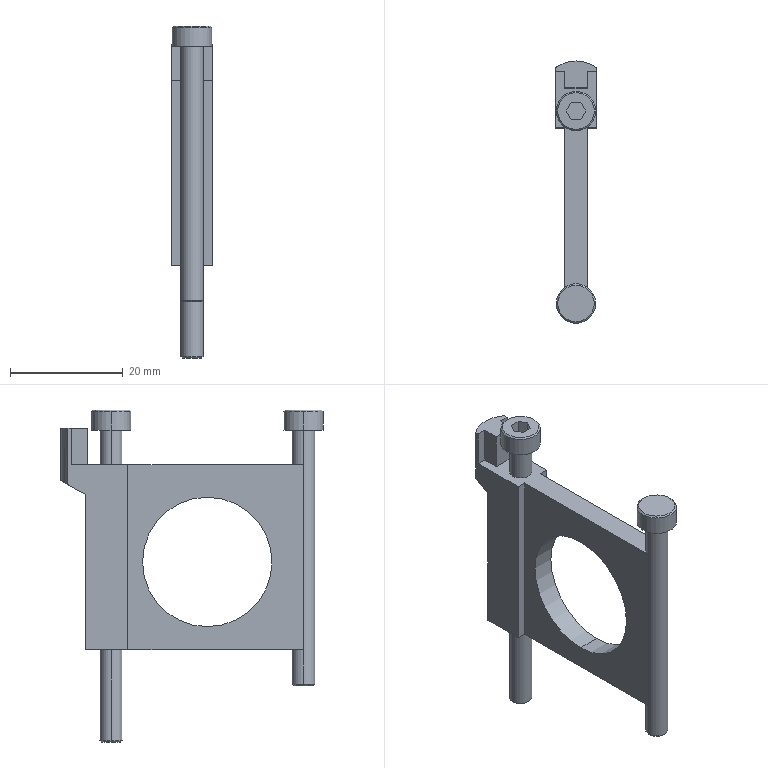Part | STEP file | Y300T_Y3035DB Interface_3 | 1 solid | 51 faces | box 7.2 x 46.6 x 59 mm | volume 5410 mm3 | plane 29 | cylinder 14 | cone 8 | commonest cylinder face diameters 4 x7 7 x4 23 x2 12 x1
STEP:
#1=CARTESIAN_POINT('',(-1.75,17.1,-32.));
#2=VERTEX_POINT('',#1);
#3=CARTESIAN_POINT('',(1.75,17.1,-32.));
#4=VERTEX_POINT('',#3);
#5=CARTESIAN_POINT('',(0.,17.1,-32.));
#6=DIRECTION('',(0.,0.,-1.));
#7=DIRECTION('',(1.,0.,0.));
#8=AXIS2_PLACEMENT_3D('',#5,#6,#7);
#9=CIRCLE('',#8,1.75);
#10=EDGE_CURVE('',#2,#4,#9,.T.);
#11=ORIENTED_EDGE('',*,*,#10,.F.);
#12=CARTESIAN_POINT('',(-2.,17.1,-31.75));
#13=VERTEX_POINT('',#12);
#14=CARTESIAN_POINT('',(-2.,17.1,-31.75));
#15=DIRECTION('',(-0.7071,0.,0.7071));
#16=VECTOR('',#15,1000.);
#17=LINE('',#14,#16);
#18=EDGE_CURVE('',#2,#13,#17,.T.);
#19=ORIENTED_EDGE('',*,*,#18,.T.);
#20=CARTESIAN_POINT('',(2.,17.1,-31.75));
#21=VERTEX_POINT('',#20);
#22=CARTESIAN_POINT('',(0.,17.1,-31.75));
#23=DIRECTION('',(0.,0.,1.));
#24=DIRECTION('',(1.,0.,0.));
#25=AXIS2_PLACEMENT_3D('',#22,#23,#24);
#26=CIRCLE('',#25,2.);
#27=EDGE_CURVE('',#21,#13,#26,.T.);
#28=ORIENTED_EDGE('',*,*,#27,.F.);
#29=CARTESIAN_POINT('',(2.,17.1,-31.75));
#30=DIRECTION('',(0.7071,0.,0.7071));
#31=VECTOR('',#30,1000.);
#32=LINE('',#29,#31);
#33=EDGE_CURVE('',#4,#21,#32,.T.);
#34=ORIENTED_EDGE('',*,*,#33,.F.);
#35=EDGE_LOOP('',(#11,#19,#28,#34));
#36=FACE_OUTER_BOUND('',#35,.T.);
#37=CARTESIAN_POINT('',(0.,17.1,-31.75));
#38=DIRECTION('',(0.,0.,1.));
#39=DIRECTION('',(1.,0.,0.));
#40=AXIS2_PLACEMENT_3D('',#37,#38,#39);
#41=CONICAL_SURFACE('',#40,2.,0.7854);
#42=ADVANCED_FACE('',(#36),#41,.T.);
#43=CARTESIAN_POINT('',(-1.75,-17.1,-22.));
#44=VERTEX_POINT('',#43);
#45=CARTESIAN_POINT('',(1.75,-17.1,-22.));
#46=VERTEX_POINT('',#45);
#47=CARTESIAN_POINT('',(0.,-17.1,-22.));
#48=DIRECTION('',(0.,0.,-1.));
#49=DIRECTION('',(1.,0.,0.));
#50=AXIS2_PLACEMENT_3D('',#47,#48,#49);
#51=CIRCLE('',#50,1.75);
#52=EDGE_CURVE('',#44,#46,#51,.T.);
#53=ORIENTED_EDGE('',*,*,#52,.F.);
#54=CARTESIAN_POINT('',(-2.,-17.1,-21.75));
#55=VERTEX_POINT('',#54);
#56=CARTESIAN_POINT('',(-2.,-17.1,-21.75));
#57=DIRECTION('',(-0.7071,0.,0.7071));
#58=VECTOR('',#57,1000.);
#59=LINE('',#56,#58);
#60=EDGE_CURVE('',#44,#55,#59,.T.);
#61=ORIENTED_EDGE('',*,*,#60,.T.);
#62=CARTESIAN_POINT('',(2.,-17.1,-21.75));
#63=VERTEX_POINT('',#62);
#64=CARTESIAN_POINT('',(0.,-17.1,-21.75));
#65=DIRECTION('',(0.,0.,1.));
#66=DIRECTION('',(1.,0.,0.));
#67=AXIS2_PLACEMENT_3D('',#64,#65,#66);
#68=CIRCLE('',#67,2.);
#69=EDGE_CURVE('',#63,#55,#68,.T.);
#70=ORIENTED_EDGE('',*,*,#69,.F.);
#71=CARTESIAN_POINT('',(2.,-17.1,-21.75));
#72=DIRECTION('',(0.7071,0.,0.7071));
#73=VECTOR('',#72,1000.);
#74=LINE('',#71,#73);
#75=EDGE_CURVE('',#46,#63,#74,.T.);
#76=ORIENTED_EDGE('',*,*,#75,.F.);
#77=EDGE_LOOP('',(#53,#61,#70,#76));
#78=FACE_OUTER_BOUND('',#77,.T.);
#79=CARTESIAN_POINT('',(0.,-17.1,-21.75));
#80=DIRECTION('',(0.,0.,1.));
#81=DIRECTION('',(1.,0.,0.));
#82=AXIS2_PLACEMENT_3D('',#79,#80,#81);
#83=CONICAL_SURFACE('',#82,2.,0.7854);
#84=ADVANCED_FACE('',(#78),#83,.T.);
#85=CARTESIAN_POINT('',(3.25,-17.1,27.));
#86=VERTEX_POINT('',#85);
#87=CARTESIAN_POINT('',(-3.25,-17.1,27.));
#88=VERTEX_POINT('',#87);
#89=CARTESIAN_POINT('',(0.,-17.1,27.));
#90=DIRECTION('',(0.,0.,1.));
#91=DIRECTION('',(-1.,0.,0.));
#92=AXIS2_PLACEMENT_3D('',#89,#90,#91);
#93=CIRCLE('',#92,3.25);
#94=EDGE_CURVE('',#86,#88,#93,.T.);
#95=ORIENTED_EDGE('',*,*,#94,.F.);
#96=CARTESIAN_POINT('',(3.5,-17.1,26.75));
#97=VERTEX_POINT('',#96);
#98=CARTESIAN_POINT('',(3.25,-17.1,27.));
#99=DIRECTION('',(0.7071,0.,-0.7071));
#100=VECTOR('',#99,1000.);
#101=LINE('',#98,#100);
#102=EDGE_CURVE('',#86,#97,#101,.T.);
#103=ORIENTED_EDGE('',*,*,#102,.T.);
#104=CARTESIAN_POINT('',(-3.5,-17.1,26.75));
#105=VERTEX_POINT('',#104);
#106=CARTESIAN_POINT('',(0.,-17.1,26.75));
#107=DIRECTION('',(0.,0.,-1.));
#108=DIRECTION('',(-1.,0.,0.));
#109=AXIS2_PLACEMENT_3D('',#106,#107,#108);
#110=CIRCLE('',#109,3.5);
#111=EDGE_CURVE('',#105,#97,#110,.T.);
#112=ORIENTED_EDGE('',*,*,#111,.F.);
#113=CARTESIAN_POINT('',(-3.25,-17.1,27.));
#114=DIRECTION('',(-0.7071,0.,-0.7071));
#115=VECTOR('',#114,1000.);
#116=LINE('',#113,#115);
#117=EDGE_CURVE('',#88,#105,#116,.T.);
#118=ORIENTED_EDGE('',*,*,#117,.F.);
#119=EDGE_LOOP('',(#95,#103,#112,#118));
#120=FACE_OUTER_BOUND('',#119,.T.);
#121=CARTESIAN_POINT('',(0.,-17.1,27.));
#122=DIRECTION('',(0.,0.,-1.));
#123=DIRECTION('',(-1.,0.,0.));
#124=AXIS2_PLACEMENT_3D('',#121,#122,#123);
#125=CONICAL_SURFACE('',#124,3.25,0.7854);
#126=ADVANCED_FACE('',(#120),#125,.T.);
#127=CARTESIAN_POINT('',(3.25,17.1,27.));
#128=VERTEX_POINT('',#127);
#129=CARTESIAN_POINT('',(-3.25,17.1,27.));
#130=VERTEX_POINT('',#129);
#131=CARTESIAN_POINT('',(0.,17.1,27.));
#132=DIRECTION('',(0.,0.,1.));
#133=DIRECTION('',(-1.,0.,0.));
#134=AXIS2_PLACEMENT_3D('',#131,#132,#133);
#135=CIRCLE('',#134,3.25);
#136=EDGE_CURVE('',#128,#130,#135,.T.);
#137=ORIENTED_EDGE('',*,*,#136,.F.);
#138=CARTESIAN_POINT('',(3.5,17.1,26.75));
#139=VERTEX_POINT('',#138);
#140=CARTESIAN_POINT('',(3.25,17.1,27.));
#141=DIRECTION('',(0.7071,0.,-0.7071));
#142=VECTOR('',#141,1000.);
#143=LINE('',#140,#142);
#144=EDGE_CURVE('',#128,#139,#143,.T.);
#145=ORIENTED_EDGE('',*,*,#144,.T.);
#146=CARTESIAN_POINT('',(-3.5,17.1,26.75));
#147=VERTEX_POINT('',#146);
#148=CARTESIAN_POINT('',(0.,17.1,26.75));
#149=DIRECTION('',(0.,0.,-1.));
#150=DIRECTION('',(-1.,0.,0.));
#151=AXIS2_PLACEMENT_3D('',#148,#149,#150);
#152=CIRCLE('',#151,3.5);
#153=EDGE_CURVE('',#147,#139,#152,.T.);
#154=ORIENTED_EDGE('',*,*,#153,.F.);
#155=CARTESIAN_POINT('',(-3.25,17.1,27.));
#156=DIRECTION('',(-0.7071,0.,-0.7071));
#157=VECTOR('',#156,1000.);
#158=LINE('',#155,#157);
#159=EDGE_CURVE('',#130,#147,#158,.T.);
#160=ORIENTED_EDGE('',*,*,#159,.F.);
#161=EDGE_LOOP('',(#137,#145,#154,#160));
#162=FACE_OUTER_BOUND('',#161,.T.);
#163=CARTESIAN_POINT('',(0.,17.1,27.));
#164=DIRECTION('',(0.,0.,-1.));
#165=DIRECTION('',(-1.,0.,0.));
#166=AXIS2_PLACEMENT_3D('',#163,#164,#165);
#167=CONICAL_SURFACE('',#166,3.25,0.7854);
#168=ADVANCED_FACE('',(#162),#167,.T.);
#169=ORIENTED_EDGE('',*,*,#69,.T.);
#170=CARTESIAN_POINT('',(-2.,-17.1,-15.6));
#171=VERTEX_POINT('',#170);
#172=CARTESIAN_POINT('',(-2.,-17.1,32.925));
#173=DIRECTION('',(0.,0.,1.));
#174=VECTOR('',#173,1000.);
#175=LINE('',#172,#174);
#176=EDGE_CURVE('',#55,#171,#175,.T.);
#177=ORIENTED_EDGE('',*,*,#176,.T.);
#178=CARTESIAN_POINT('',(2.,-17.1,-15.6));
#179=VERTEX_POINT('',#178);
#180=CARTESIAN_POINT('',(0.,-17.1,-15.6));
#181=DIRECTION('',(0.,0.,-1.));
#182=DIRECTION('',(0.,-1.,0.));
#183=AXIS2_PLACEMENT_3D('',#180,#181,#182);
#184=CIRCLE('',#183,2.);
#185=EDGE_CURVE('',#171,#179,#184,.T.);
#186=ORIENTED_EDGE('',*,*,#185,.T.);
#187=CARTESIAN_POINT('',(2.,-17.1,32.925));
#188=DIRECTION('',(0.,0.,1.));
#189=VECTOR('',#188,1000.);
#190=LINE('',#187,#189);
#191=EDGE_CURVE('',#63,#179,#190,.T.);
#192=ORIENTED_EDGE('',*,*,#191,.F.);
#193=EDGE_LOOP('',(#169,#177,#186,#192));
#194=FACE_OUTER_BOUND('',#193,.T.);
#195=CARTESIAN_POINT('',(0.,-17.1,32.925));
#196=DIRECTION('',(0.,0.,1.));
#197=DIRECTION('',(1.,0.,0.));
#198=AXIS2_PLACEMENT_3D('',#195,#196,#197);
#199=CYLINDRICAL_SURFACE('',#198,2.);
#200=ADVANCED_FACE('',(#194),#199,.T.);
#201=CARTESIAN_POINT('',(2.,-17.1,17.3));
#202=VERTEX_POINT('',#201);
#203=CARTESIAN_POINT('',(-2.,-17.1,17.3));
#204=VERTEX_POINT('',#203);
#205=CARTESIAN_POINT('',(0.,-17.1,17.3));
#206=DIRECTION('',(0.,0.,1.));
#207=DIRECTION('',(-1.,0.,0.));
#208=AXIS2_PLACEMENT_3D('',#205,#206,#207);
#209=CIRCLE('',#208,2.);
#210=EDGE_CURVE('',#202,#204,#209,.T.);
#211=ORIENTED_EDGE('',*,*,#210,.T.);
#212=CARTESIAN_POINT('',(-2.,-17.1,23.4));
#213=VERTEX_POINT('',#212);
#214=CARTESIAN_POINT('',(-2.,-17.1,32.925));
#215=DIRECTION('',(0.,0.,1.));
#216=VECTOR('',#215,1000.);
#217=LINE('',#214,#216);
#218=EDGE_CURVE('',#204,#213,#217,.T.);
#219=ORIENTED_EDGE('',*,*,#218,.T.);
#220=CARTESIAN_POINT('',(2.,-17.1,23.4));
#221=VERTEX_POINT('',#220);
#222=CARTESIAN_POINT('',(0.,-17.1,23.4));
#223=DIRECTION('',(0.,0.,1.));
#224=DIRECTION('',(1.,0.,0.));
#225=AXIS2_PLACEMENT_3D('',#222,#223,#224);
#226=CIRCLE('',#225,2.);
#227=EDGE_CURVE('',#221,#213,#226,.T.);
#228=ORIENTED_EDGE('',*,*,#227,.F.);
#229=CARTESIAN_POINT('',(2.,-17.1,32.925));
#230=DIRECTION('',(0.,0.,1.));
#231=VECTOR('',#230,1000.);
#232=LINE('',#229,#231);
#233=EDGE_CURVE('',#202,#221,#232,.T.);
#234=ORIENTED_EDGE('',*,*,#233,.F.);
#235=EDGE_LOOP('',(#211,#219,#228,#234));
#236=FACE_OUTER_BOUND('',#235,.T.);
#237=CARTESIAN_POINT('',(0.,-17.1,32.925));
#238=DIRECTION('',(0.,0.,1.));
#239=DIRECTION('',(1.,0.,0.));
#240=AXIS2_PLACEMENT_3D('',#237,#238,#239);
#241=CYLINDRICAL_SURFACE('',#240,2.);
#242=ADVANCED_FACE('',(#236),#241,.T.);
#243=CARTESIAN_POINT('',(3.5,-17.1,23.4));
#244=VERTEX_POINT('',#243);
#245=CARTESIAN_POINT('',(-3.5,-17.1,23.4));
#246=VERTEX_POINT('',#245);
#247=CARTESIAN_POINT('',(0.,-17.1,23.4));
#248=DIRECTION('',(0.,0.,1.));
#249=DIRECTION('',(1.,0.,0.));
#250=AXIS2_PLACEMENT_3D('',#247,#248,#249);
#251=CIRCLE('',#250,3.5);
#252=EDGE_CURVE('',#244,#246,#251,.T.);
#253=ORIENTED_EDGE('',*,*,#252,.T.);
#254=CARTESIAN_POINT('',(-3.5,-17.1,32.925));
#255=DIRECTION('',(0.,0.,1.));
#256=VECTOR('',#255,1000.);
#257=LINE('',#254,#256);
#258=EDGE_CURVE('',#246,#105,#257,.T.);
#259=ORIENTED_EDGE('',*,*,#258,.T.);
#260=ORIENTED_EDGE('',*,*,#111,.T.);
#261=CARTESIAN_POINT('',(3.5,-17.1,32.925));
#262=DIRECTION('',(0.,0.,1.));
#263=VECTOR('',#262,1000.);
#264=LINE('',#261,#263);
#265=EDGE_CURVE('',#244,#97,#264,.T.);
#266=ORIENTED_EDGE('',*,*,#265,.F.);
#267=EDGE_LOOP('',(#253,#259,#260,#266));
#268=FACE_OUTER_BOUND('',#267,.T.);
#269=CARTESIAN_POINT('',(0.,-17.1,32.925));
#270=DIRECTION('',(0.,0.,1.));
#271=DIRECTION('',(1.,0.,0.));
#272=AXIS2_PLACEMENT_3D('',#269,#270,#271);
#273=CYLINDRICAL_SURFACE('',#272,3.5);
#274=ADVANCED_FACE('',(#268),#273,.T.);
#275=ORIENTED_EDGE('',*,*,#27,.T.);
#276=CARTESIAN_POINT('',(-2.,17.1,-15.6));
#277=VERTEX_POINT('',#276);
#278=CARTESIAN_POINT('',(-2.,17.1,35.151));
#279=DIRECTION('',(0.,0.,1.));
#280=VECTOR('',#279,1000.);
#281=LINE('',#278,#280);
#282=EDGE_CURVE('',#13,#277,#281,.T.);
#283=ORIENTED_EDGE('',*,*,#282,.T.);
#284=CARTESIAN_POINT('',(2.,17.1,-15.6));
#285=VERTEX_POINT('',#284);
#286=CARTESIAN_POINT('',(0.,17.1,-15.6));
#287=DIRECTION('',(0.,0.,-1.));
#288=DIRECTION('',(0.,-1.,0.));
#289=AXIS2_PLACEMENT_3D('',#286,#287,#288);
#290=CIRCLE('',#289,2.);
#291=EDGE_CURVE('',#277,#285,#290,.T.);
#292=ORIENTED_EDGE('',*,*,#291,.T.);
#293=CARTESIAN_POINT('',(2.,17.1,35.151));
#294=DIRECTION('',(0.,0.,1.));
#295=VECTOR('',#294,1000.);
#296=LINE('',#293,#295);
#297=EDGE_CURVE('',#21,#285,#296,.T.);
#298=ORIENTED_EDGE('',*,*,#297,.F.);
#299=EDGE_LOOP('',(#275,#283,#292,#298));
#300=FACE_OUTER_BOUND('',#299,.T.);
#301=CARTESIAN_POINT('',(0.,17.1,35.151));
#302=DIRECTION('',(0.,0.,1.));
#303=DIRECTION('',(1.,0.,0.));
#304=AXIS2_PLACEMENT_3D('',#301,#302,#303);
#305=CYLINDRICAL_SURFACE('',#304,2.);
#306=ADVANCED_FACE('',(#300),#305,.T.);
#307=CARTESIAN_POINT('',(2.,17.1,17.3));
#308=VERTEX_POINT('',#307);
#309=CARTESIAN_POINT('',(-2.,17.1,17.3));
#310=VERTEX_POINT('',#309);
#311=CARTESIAN_POINT('',(0.,17.1,17.3));
#312=DIRECTION('',(0.,0.,1.));
#313=DIRECTION('',(-1.,0.,0.));
#314=AXIS2_PLACEMENT_3D('',#311,#312,#313);
#315=CIRCLE('',#314,2.);
#316=EDGE_CURVE('',#308,#310,#315,.T.);
#317=ORIENTED_EDGE('',*,*,#316,.T.);
#318=CARTESIAN_POINT('',(-2.,17.1,23.4));
#319=VERTEX_POINT('',#318);
#320=CARTESIAN_POINT('',(-2.,17.1,35.151));
#321=DIRECTION('',(0.,0.,1.));
#322=VECTOR('',#321,1000.);
#323=LINE('',#320,#322);
#324=EDGE_CURVE('',#310,#319,#323,.T.);
#325=ORIENTED_EDGE('',*,*,#324,.T.);
#326=CARTESIAN_POINT('',(2.,17.1,23.4));
#327=VERTEX_POINT('',#326);
#328=CARTESIAN_POINT('',(0.,17.1,23.4));
#329=DIRECTION('',(0.,0.,1.));
#330=DIRECTION('',(1.,0.,0.));
#331=AXIS2_PLACEMENT_3D('',#328,#329,#330);
#332=CIRCLE('',#331,2.);
#333=EDGE_CURVE('',#327,#319,#332,.T.);
#334=ORIENTED_EDGE('',*,*,#333,.F.);
#335=CARTESIAN_POINT('',(2.,17.1,35.151));
#336=DIRECTION('',(0.,0.,1.));
#337=VECTOR('',#336,1000.);
#338=LINE('',#335,#337);
#339=EDGE_CURVE('',#308,#327,#338,.T.);
#340=ORIENTED_EDGE('',*,*,#339,.F.);
#341=EDGE_LOOP('',(#317,#325,#334,#340));
#342=FACE_OUTER_BOUND('',#341,.T.);
#343=CARTESIAN_POINT('',(0.,17.1,35.151));
#344=DIRECTION('',(0.,0.,1.));
#345=DIRECTION('',(1.,0.,0.));
#346=AXIS2_PLACEMENT_3D('',#343,#344,#345);
#347=CYLINDRICAL_SURFACE('',#346,2.);
#348=ADVANCED_FACE('',(#342),#347,.T.);
#349=CARTESIAN_POINT('',(3.5,17.1,23.4));
#350=VERTEX_POINT('',#349);
#351=CARTESIAN_POINT('',(-3.5,17.1,23.4));
#352=VERTEX_POINT('',#351);
#353=CARTESIAN_POINT('',(0.,17.1,23.4));
#354=DIRECTION('',(0.,0.,1.));
#355=DIRECTION('',(1.,0.,0.));
#356=AXIS2_PLACEMENT_3D('',#353,#354,#355);
#357=CIRCLE('',#356,3.5);
#358=EDGE_CURVE('',#350,#352,#357,.T.);
#359=ORIENTED_EDGE('',*,*,#358,.T.);
#360=CARTESIAN_POINT('',(-3.5,17.1,35.151));
#361=DIRECTION('',(0.,0.,1.));
#362=VECTOR('',#361,1000.);
#363=LINE('',#360,#362);
#364=EDGE_CURVE('',#352,#147,#363,.T.);
#365=ORIENTED_EDGE('',*,*,#364,.T.);
#366=ORIENTED_EDGE('',*,*,#153,.T.);
#367=CARTESIAN_POINT('',(3.5,17.1,35.151));
#368=DIRECTION('',(0.,0.,1.));
#369=VECTOR('',#368,1000.);
#370=LINE('',#367,#369);
#371=EDGE_CURVE('',#350,#139,#370,.T.);
#372=ORIENTED_EDGE('',*,*,#371,.F.);
#373=EDGE_LOOP('',(#359,#365,#366,#372));
#374=FACE_OUTER_BOUND('',#373,.T.);
#375=CARTESIAN_POINT('',(0.,17.1,35.151));
#376=DIRECTION('',(0.,0.,1.));
#377=DIRECTION('',(1.,0.,0.));
#378=AXIS2_PLACEMENT_3D('',#375,#376,#377);
#379=CYLINDRICAL_SURFACE('',#378,3.5);
#380=ADVANCED_FACE('',(#374),#379,.T.);
#381=CARTESIAN_POINT('',(-2.,0.,-11.5));
#382=VERTEX_POINT('',#381);
#383=CARTESIAN_POINT('',(-2.,0.,11.5));
#384=VERTEX_POINT('',#383);
#385=CARTESIAN_POINT('',(-2.,0.,0.));
#386=DIRECTION('',(-1.,0.,0.));
#387=DIRECTION('',(0.,0.,1.));
#388=AXIS2_PLACEMENT_3D('',#385,#386,#387);
#389=CIRCLE('',#388,11.5);
#390=EDGE_CURVE('',#382,#384,#389,.T.);
#391=ORIENTED_EDGE('',*,*,#390,.T.);
#392=CARTESIAN_POINT('',(2.,0.,11.5));
#393=VERTEX_POINT('',#392);
#394=CARTESIAN_POINT('',(-3.6,0.,11.5));
#395=DIRECTION('',(1.,0.,0.));
#396=VECTOR('',#395,1000.);
#397=LINE('',#394,#396);
#398=EDGE_CURVE('',#384,#393,#397,.T.);
#399=ORIENTED_EDGE('',*,*,#398,.T.);
#400=CARTESIAN_POINT('',(2.,0.,-11.5));
#401=VERTEX_POINT('',#400);
#402=CARTESIAN_POINT('',(2.,0.,0.));
#403=DIRECTION('',(-1.,0.,0.));
#404=DIRECTION('',(0.,0.,1.));
#405=AXIS2_PLACEMENT_3D('',#402,#403,#404);
#406=CIRCLE('',#405,11.5);
#407=EDGE_CURVE('',#401,#393,#406,.T.);
#408=ORIENTED_EDGE('',*,*,#407,.F.);
#409=CARTESIAN_POINT('',(-3.6,0.,-11.5));
#410=DIRECTION('',(1.,0.,0.));
#411=VECTOR('',#410,1000.);
#412=LINE('',#409,#411);
#413=EDGE_CURVE('',#382,#401,#412,.T.);
#414=ORIENTED_EDGE('',*,*,#413,.F.);
#415=EDGE_LOOP('',(#391,#399,#408,#414));
#416=FACE_OUTER_BOUND('',#415,.T.);
#417=CARTESIAN_POINT('',(-3.6,0.,0.));
#418=DIRECTION('',(1.,0.,0.));
#419=DIRECTION('',(0.,0.,-1.));
#420=AXIS2_PLACEMENT_3D('',#417,#418,#419);
#421=CYLINDRICAL_SURFACE('',#420,11.5);
#422=ADVANCED_FACE('',(#416),#421,.F.);
#423=CARTESIAN_POINT('',(0.,17.1,-15.6));
#424=DIRECTION('',(0.,0.,-1.));
#425=DIRECTION('',(0.,-1.,0.));
#426=AXIS2_PLACEMENT_3D('',#423,#424,#425);
#427=CIRCLE('',#426,2.);
#428=EDGE_CURVE('',#285,#277,#427,.T.);
#429=ORIENTED_EDGE('',*,*,#428,.F.);
#430=ORIENTED_EDGE('',*,*,#291,.F.);
#431=EDGE_LOOP('',(#429,#430));
#432=FACE_BOUND('',#431,.T.);
#433=ORIENTED_EDGE('',*,*,#185,.F.);
#434=CARTESIAN_POINT('',(-2.,14.1,-15.6));
#435=VERTEX_POINT('',#434);
#436=CARTESIAN_POINT('',(-2.,-17.1,-15.6));
#437=DIRECTION('',(0.,1.,0.));
#438=VECTOR('',#437,1000.);
#439=LINE('',#436,#438);
#440=EDGE_CURVE('',#171,#435,#439,.T.);
#441=ORIENTED_EDGE('',*,*,#440,.T.);
#442=CARTESIAN_POINT('',(-3.6,14.1,-15.6));
#443=VERTEX_POINT('',#442);
#444=CARTESIAN_POINT('',(3.6,14.1,-15.6));
#445=DIRECTION('',(-1.,0.,0.));
#446=VECTOR('',#445,1000.);
#447=LINE('',#444,#446);
#448=EDGE_CURVE('',#435,#443,#447,.T.);
#449=ORIENTED_EDGE('',*,*,#448,.T.);
#450=CARTESIAN_POINT('',(-3.6,21.7,-15.6));
#451=VERTEX_POINT('',#450);
#452=CARTESIAN_POINT('',(-3.6,14.1,-15.6));
#453=DIRECTION('',(0.,1.,0.));
#454=VECTOR('',#453,1000.);
#455=LINE('',#452,#454);
#456=EDGE_CURVE('',#443,#451,#455,.T.);
#457=ORIENTED_EDGE('',*,*,#456,.T.);
#458=CARTESIAN_POINT('',(3.6,21.7,-15.6));
#459=VERTEX_POINT('',#458);
#460=CARTESIAN_POINT('',(76.046,21.7,-15.6));
#461=DIRECTION('',(-1.,0.,0.));
#462=VECTOR('',#461,1000.);
#463=LINE('',#460,#462);
#464=EDGE_CURVE('',#459,#451,#463,.T.);
#465=ORIENTED_EDGE('',*,*,#464,.F.);
#466=CARTESIAN_POINT('',(3.6,14.1,-15.6));
#467=VERTEX_POINT('',#466);
#468=CARTESIAN_POINT('',(3.6,14.1,-15.6));
#469=DIRECTION('',(0.,-1.,0.));
#470=VECTOR('',#469,1000.);
#471=LINE('',#468,#470);
#472=EDGE_CURVE('',#459,#467,#471,.T.);
#473=ORIENTED_EDGE('',*,*,#472,.T.);
#474=CARTESIAN_POINT('',(2.,14.1,-15.6));
#475=VERTEX_POINT('',#474);
#476=CARTESIAN_POINT('',(3.6,14.1,-15.6));
#477=DIRECTION('',(-1.,0.,0.));
#478=VECTOR('',#477,1000.);
#479=LINE('',#476,#478);
#480=EDGE_CURVE('',#467,#475,#479,.T.);
#481=ORIENTED_EDGE('',*,*,#480,.T.);
#482=CARTESIAN_POINT('',(2.,-17.1,-15.6));
#483=DIRECTION('',(0.,1.,0.));
#484=VECTOR('',#483,1000.);
#485=LINE('',#482,#484);
#486=EDGE_CURVE('',#179,#475,#485,.T.);
#487=ORIENTED_EDGE('',*,*,#486,.F.);
#488=EDGE_LOOP('',(#433,#441,#449,#457,#465,#473,#481,#487));
#489=FACE_OUTER_BOUND('',#488,.T.);
#490=CARTESIAN_POINT('',(2.,-17.1,-15.6));
#491=DIRECTION('',(0.,0.,1.));
#492=DIRECTION('',(0.,-1.,0.));
#493=AXIS2_PLACEMENT_3D('',#490,#491,#492);
#494=PLANE('',#493);
#495=ADVANCED_FACE('',(#432,#489),#494,.F.);
#496=ORIENTED_EDGE('',*,*,#316,.F.);
#497=CARTESIAN_POINT('',(0.,17.1,17.3));
#498=DIRECTION('',(0.,0.,1.));
#499=DIRECTION('',(-1.,0.,0.));
#500=AXIS2_PLACEMENT_3D('',#497,#498,#499);
#501=CIRCLE('',#500,2.);
#502=EDGE_CURVE('',#310,#308,#501,.T.);
#503=ORIENTED_EDGE('',*,*,#502,.F.);
#504=EDGE_LOOP('',(#496,#503));
#505=FACE_BOUND('',#504,.T.);
#506=ORIENTED_EDGE('',*,*,#210,.F.);
#507=CARTESIAN_POINT('',(2.,14.1,17.3));
#508=VERTEX_POINT('',#507);
#509=CARTESIAN_POINT('',(2.,-17.1,17.3));
#510=DIRECTION('',(0.,-1.,0.));
#511=VECTOR('',#510,1000.);
#512=LINE('',#509,#511);
#513=EDGE_CURVE('',#508,#202,#512,.T.);
#514=ORIENTED_EDGE('',*,*,#513,.F.);
#515=CARTESIAN_POINT('',(3.6,14.1,17.3));
#516=VERTEX_POINT('',#515);
#517=CARTESIAN_POINT('',(-3.6,14.1,17.3));
#518=DIRECTION('',(1.,0.,0.));
#519=VECTOR('',#518,1000.);
#520=LINE('',#517,#519);
#521=EDGE_CURVE('',#508,#516,#520,.T.);
#522=ORIENTED_EDGE('',*,*,#521,.T.);
#523=CARTESIAN_POINT('',(3.6,24.1,17.3));
#524=VERTEX_POINT('',#523);
#525=CARTESIAN_POINT('',(3.6,24.1,17.3));
#526=DIRECTION('',(0.,1.,0.));
#527=VECTOR('',#526,1000.);
#528=LINE('',#525,#527);
#529=EDGE_CURVE('',#516,#524,#528,.T.);
#530=ORIENTED_EDGE('',*,*,#529,.T.);
#531=CARTESIAN_POINT('',(2.,24.1,17.3));
#532=VERTEX_POINT('',#531);
#533=CARTESIAN_POINT('',(3.6,24.1,17.3));
#534=DIRECTION('',(-1.,0.,0.));
#535=VECTOR('',#534,1000.);
#536=LINE('',#533,#535);
#537=EDGE_CURVE('',#524,#532,#536,.T.);
#538=ORIENTED_EDGE('',*,*,#537,.T.);
#539=CARTESIAN_POINT('',(2.,21.2,17.3));
#540=VERTEX_POINT('',#539);
#541=CARTESIAN_POINT('',(2.,24.1,17.3));
#542=DIRECTION('',(0.,-1.,0.));
#543=VECTOR('',#542,1000.);
#544=LINE('',#541,#543);
#545=EDGE_CURVE('',#532,#540,#544,.T.);
#546=ORIENTED_EDGE('',*,*,#545,.T.);
#547=CARTESIAN_POINT('',(-2.,21.2,17.3));
#548=VERTEX_POINT('',#547);
#549=CARTESIAN_POINT('',(-2.,21.2,17.3));
#550=DIRECTION('',(-1.,0.,0.));
#551=VECTOR('',#550,1000.);
#552=LINE('',#549,#551);
#553=EDGE_CURVE('',#540,#548,#552,.T.);
#554=ORIENTED_EDGE('',*,*,#553,.T.);
#555=CARTESIAN_POINT('',(-2.,24.1,17.3));
#556=VERTEX_POINT('',#555);
#557=CARTESIAN_POINT('',(-2.,24.1,17.3));
#558=DIRECTION('',(0.,1.,0.));
#559=VECTOR('',#558,1000.);
#560=LINE('',#557,#559);
#561=EDGE_CURVE('',#548,#556,#560,.T.);
#562=ORIENTED_EDGE('',*,*,#561,.T.);
#563=CARTESIAN_POINT('',(-3.6,24.1,17.3));
#564=VERTEX_POINT('',#563);
#565=CARTESIAN_POINT('',(-3.6,24.1,17.3));
#566=DIRECTION('',(-1.,0.,0.));
#567=VECTOR('',#566,1000.);
#568=LINE('',#565,#567);
#569=EDGE_CURVE('',#556,#564,#568,.T.);
#570=ORIENTED_EDGE('',*,*,#569,.T.);
#571=CARTESIAN_POINT('',(-3.6,14.1,17.3));
#572=VERTEX_POINT('',#571);
#573=CARTESIAN_POINT('',(-3.6,24.1,17.3));
#574=DIRECTION('',(0.,-1.,0.));
#575=VECTOR('',#574,1000.);
#576=LINE('',#573,#575);
#577=EDGE_CURVE('',#564,#572,#576,.T.);
#578=ORIENTED_EDGE('',*,*,#577,.T.);
#579=CARTESIAN_POINT('',(-2.,14.1,17.3));
#580=VERTEX_POINT('',#579);
#581=CARTESIAN_POINT('',(-3.6,14.1,17.3));
#582=DIRECTION('',(1.,0.,0.));
#583=VECTOR('',#582,1000.);
#584=LINE('',#581,#583);
#585=EDGE_CURVE('',#572,#580,#584,.T.);
#586=ORIENTED_EDGE('',*,*,#585,.T.);
#587=CARTESIAN_POINT('',(-2.,-17.1,17.3));
#588=DIRECTION('',(0.,-1.,0.));
#589=VECTOR('',#588,1000.);
#590=LINE('',#587,#589);
#591=EDGE_CURVE('',#580,#204,#590,.T.);
#592=ORIENTED_EDGE('',*,*,#591,.T.);
#593=EDGE_LOOP('',(#506,#514,#522,#530,#538,#546,#554,#562,#570,#578,#586,#592));
#594=FACE_OUTER_BOUND('',#593,.T.);
#595=CARTESIAN_POINT('',(2.,-17.1,17.3));
#596=DIRECTION('',(0.,0.,-1.));
#597=DIRECTION('',(-1.,0.,0.));
#598=AXIS2_PLACEMENT_3D('',#595,#596,#597);
#599=PLANE('',#598);
#600=ADVANCED_FACE('',(#505,#594),#599,.F.);
#601=CARTESIAN_POINT('',(3.6,24.8,23.8));
#602=VERTEX_POINT('',#601);
#603=CARTESIAN_POINT('',(3.6,24.1,23.8));
#604=VERTEX_POINT('',#603);
#605=CARTESIAN_POINT('',(3.6,14.1,23.8));
#606=DIRECTION('',(0.,-1.,0.));
#607=VECTOR('',#606,1000.);
#608=LINE('',#605,#607);
#609=EDGE_CURVE('',#602,#604,#608,.T.);
#610=ORIENTED_EDGE('',*,*,#609,.T.);
#611=CARTESIAN_POINT('',(3.6,24.1,23.8));
#612=DIRECTION('',(0.,0.,-1.));
#613=VECTOR('',#612,1000.);
#614=LINE('',#611,#613);
#615=EDGE_CURVE('',#604,#524,#614,.T.);
#616=ORIENTED_EDGE('',*,*,#615,.T.);
#617=ORIENTED_EDGE('',*,*,#529,.F.);
#618=CARTESIAN_POINT('',(3.6,14.1,23.8));
#619=DIRECTION('',(0.,0.,-1.));
#620=VECTOR('',#619,1000.);
#621=LINE('',#618,#620);
#622=EDGE_CURVE('',#516,#467,#621,.T.);
#623=ORIENTED_EDGE('',*,*,#622,.T.);
#624=ORIENTED_EDGE('',*,*,#472,.F.);
#625=CARTESIAN_POINT('',(3.6,21.7,12.));
#626=VERTEX_POINT('',#625);
#627=CARTESIAN_POINT('',(3.6,21.7,23.8));
#628=DIRECTION('',(0.,0.,1.));
#629=VECTOR('',#628,1000.);
#630=LINE('',#627,#629);
#631=EDGE_CURVE('',#459,#626,#630,.T.);
#632=ORIENTED_EDGE('',*,*,#631,.T.);
#633=CARTESIAN_POINT('',(3.6,24.8,13.79));
#634=VERTEX_POINT('',#633);
#635=CARTESIAN_POINT('',(3.6,21.11,11.659));
#636=DIRECTION('',(0.,0.866,0.5));
#637=VECTOR('',#636,1000.);
#638=LINE('',#635,#637);
#639=EDGE_CURVE('',#626,#634,#638,.T.);
#640=ORIENTED_EDGE('',*,*,#639,.T.);
#641=CARTESIAN_POINT('',(3.6,24.8,23.8));
#642=DIRECTION('',(0.,0.,-1.));
#643=VECTOR('',#642,1000.);
#644=LINE('',#641,#643);
#645=EDGE_CURVE('',#602,#634,#644,.T.);
#646=ORIENTED_EDGE('',*,*,#645,.F.);
#647=EDGE_LOOP('',(#610,#616,#617,#623,#624,#632,#640,#646));
#648=FACE_OUTER_BOUND('',#647,.T.);
#649=CARTESIAN_POINT('',(3.6,14.1,23.8));
#650=DIRECTION('',(1.,0.,0.));
#651=DIRECTION('',(0.,0.,-1.));
#652=AXIS2_PLACEMENT_3D('',#649,#650,#651);
#653=PLANE('',#652);
#654=ADVANCED_FACE('',(#648),#653,.T.);
#655=ORIENTED_EDGE('',*,*,#577,.F.);
#656=CARTESIAN_POINT('',(-3.6,24.1,23.8));
#657=VERTEX_POINT('',#656);
#658=CARTESIAN_POINT('',(-3.6,24.1,23.8));
#659=DIRECTION('',(0.,0.,-1.));
#660=VECTOR('',#659,1000.);
#661=LINE('',#658,#660);
#662=EDGE_CURVE('',#657,#564,#661,.T.);
#663=ORIENTED_EDGE('',*,*,#662,.F.);
#664=CARTESIAN_POINT('',(-3.6,24.8,23.8));
#665=VERTEX_POINT('',#664);
#666=CARTESIAN_POINT('',(-3.6,14.1,23.8));
#667=DIRECTION('',(0.,1.,0.));
#668=VECTOR('',#667,1000.);
#669=LINE('',#666,#668);
#670=EDGE_CURVE('',#657,#665,#669,.T.);
#671=ORIENTED_EDGE('',*,*,#670,.T.);
#672=CARTESIAN_POINT('',(-3.6,24.8,13.79));
#673=VERTEX_POINT('',#672);
#674=CARTESIAN_POINT('',(-3.6,24.8,23.8));
#675=DIRECTION('',(0.,0.,-1.));
#676=VECTOR('',#675,1000.);
#677=LINE('',#674,#676);
#678=EDGE_CURVE('',#665,#673,#677,.T.);
#679=ORIENTED_EDGE('',*,*,#678,.T.);
#680=CARTESIAN_POINT('',(-3.6,21.7,12.));
#681=VERTEX_POINT('',#680);
#682=CARTESIAN_POINT('',(-3.6,21.11,11.659));
#683=DIRECTION('',(0.,-0.866,-0.5));
#684=VECTOR('',#683,1000.);
#685=LINE('',#682,#684);
#686=EDGE_CURVE('',#673,#681,#685,.T.);
#687=ORIENTED_EDGE('',*,*,#686,.T.);
#688=CARTESIAN_POINT('',(-3.6,21.7,23.8));
#689=DIRECTION('',(0.,0.,-1.));
#690=VECTOR('',#689,1000.);
#691=LINE('',#688,#690);
#692=EDGE_CURVE('',#681,#451,#691,.T.);
#693=ORIENTED_EDGE('',*,*,#692,.T.);
#694=ORIENTED_EDGE('',*,*,#456,.F.);
#695=CARTESIAN_POINT('',(-3.6,14.1,23.8));
#696=DIRECTION('',(0.,0.,-1.));
#697=VECTOR('',#696,1000.);
#698=LINE('',#695,#697);
#699=EDGE_CURVE('',#572,#443,#698,.T.);
#700=ORIENTED_EDGE('',*,*,#699,.F.);
#701=EDGE_LOOP('',(#655,#663,#671,#679,#687,#693,#694,#700));
#702=FACE_OUTER_BOUND('',#701,.T.);
#703=CARTESIAN_POINT('',(-3.6,14.1,23.8));
#704=DIRECTION('',(-1.,0.,0.));
#705=DIRECTION('',(0.,0.,1.));
#706=AXIS2_PLACEMENT_3D('',#703,#704,#705);
#707=PLANE('',#706);
#708=ADVANCED_FACE('',(#702),#707,.T.);
#709=ORIENTED_EDGE('',*,*,#585,.F.);
#710=ORIENTED_EDGE('',*,*,#699,.T.);
#711=ORIENTED_EDGE('',*,*,#448,.F.);
#712=CARTESIAN_POINT('',(-2.,14.1,17.3));
#713=DIRECTION('',(0.,0.,1.));
#714=VECTOR('',#713,1000.);
#715=LINE('',#712,#714);
#716=EDGE_CURVE('',#435,#580,#715,.T.);
#717=ORIENTED_EDGE('',*,*,#716,.T.);
#718=EDGE_LOOP('',(#709,#710,#711,#717));
#719=FACE_OUTER_BOUND('',#718,.T.);
#720=CARTESIAN_POINT('',(3.6,14.1,23.8));
#721=DIRECTION('',(0.,-1.,0.));
#722=DIRECTION('',(0.,0.,-1.));
#723=AXIS2_PLACEMENT_3D('',#720,#721,#722);
#724=PLANE('',#723);
#725=ADVANCED_FACE('',(#719),#724,.T.);
#726=ORIENTED_EDGE('',*,*,#670,.F.);
#727=CARTESIAN_POINT('',(-2.,24.1,23.8));
#728=VERTEX_POINT('',#727);
#729=CARTESIAN_POINT('',(-3.6,24.1,23.8));
#730=DIRECTION('',(-1.,0.,0.));
#731=VECTOR('',#730,1000.);
#732=LINE('',#729,#731);
#733=EDGE_CURVE('',#728,#657,#732,.T.);
#734=ORIENTED_EDGE('',*,*,#733,.F.);
#735=CARTESIAN_POINT('',(-2.,21.2,23.8));
#736=VERTEX_POINT('',#735);
#737=CARTESIAN_POINT('',(-2.,24.1,23.8));
#738=DIRECTION('',(0.,1.,0.));
#739=VECTOR('',#738,1000.);
#740=LINE('',#737,#739);
#741=EDGE_CURVE('',#736,#728,#740,.T.);
#742=ORIENTED_EDGE('',*,*,#741,.F.);
#743=CARTESIAN_POINT('',(2.,21.2,23.8));
#744=VERTEX_POINT('',#743);
#745=CARTESIAN_POINT('',(-2.,21.2,23.8));
#746=DIRECTION('',(-1.,0.,0.));
#747=VECTOR('',#746,1000.);
#748=LINE('',#745,#747);
#749=EDGE_CURVE('',#744,#736,#748,.T.);
#750=ORIENTED_EDGE('',*,*,#749,.F.);
#751=CARTESIAN_POINT('',(2.,24.1,23.8));
#752=VERTEX_POINT('',#751);
#753=CARTESIAN_POINT('',(2.,24.1,23.8));
#754=DIRECTION('',(0.,-1.,0.));
#755=VECTOR('',#754,1000.);
#756=LINE('',#753,#755);
#757=EDGE_CURVE('',#752,#744,#756,.T.);
#758=ORIENTED_EDGE('',*,*,#757,.F.);
#759=CARTESIAN_POINT('',(3.6,24.1,23.8));
#760=DIRECTION('',(-1.,0.,0.));
#761=VECTOR('',#760,1000.);
#762=LINE('',#759,#761);
#763=EDGE_CURVE('',#604,#752,#762,.T.);
#764=ORIENTED_EDGE('',*,*,#763,.F.);
#765=ORIENTED_EDGE('',*,*,#609,.F.);
#766=CARTESIAN_POINT('',(0.,20.,23.8));
#767=DIRECTION('',(0.,0.,-1.));
#768=DIRECTION('',(1.,0.,0.));
#769=AXIS2_PLACEMENT_3D('',#766,#767,#768);
#770=CIRCLE('',#769,6.);
#771=EDGE_CURVE('',#665,#602,#770,.T.);
#772=ORIENTED_EDGE('',*,*,#771,.F.);
#773=EDGE_LOOP('',(#726,#734,#742,#750,#758,#764,#765,#772));
#774=FACE_OUTER_BOUND('',#773,.T.);
#775=CARTESIAN_POINT('',(0.,20.,23.8));
#776=DIRECTION('',(0.,0.,1.));
#777=DIRECTION('',(1.,0.,0.));
#778=AXIS2_PLACEMENT_3D('',#775,#776,#777);
#779=PLANE('',#778);
#780=ADVANCED_FACE('',(#774),#779,.T.);
#781=ORIENTED_EDGE('',*,*,#645,.T.);
#782=CARTESIAN_POINT('',(3.6,24.8,13.79));
#783=CARTESIAN_POINT('',(1.385,26.462,14.749));
#784=CARTESIAN_POINT('',(-1.385,26.462,14.749));
#785=CARTESIAN_POINT('',(-3.6,24.8,13.79));
#786=(BOUNDED_CURVE()B_SPLINE_CURVE(3,(#782,#783,#784,#785),.UNSPECIFIED.,.F.,.F.)B_SPLINE_CURVE_WITH_KNOTS((4,4),(2.498,3.785),.UNSPECIFIED.)CURVE()GEOMETRIC_REPRESENTATION_ITEM()RATIONAL_B_SPLINE_CURVE((1.,0.8667,0.8667,1.))REPRESENTATION_ITEM(''));
#787=EDGE_CURVE('',#634,#673,#786,.T.);
#788=ORIENTED_EDGE('',*,*,#787,.T.);
#789=ORIENTED_EDGE('',*,*,#678,.F.);
#790=ORIENTED_EDGE('',*,*,#771,.T.);
#791=EDGE_LOOP('',(#781,#788,#789,#790));
#792=FACE_OUTER_BOUND('',#791,.T.);
#793=CARTESIAN_POINT('',(0.,20.,23.8));
#794=DIRECTION('',(0.,0.,-1.));
#795=DIRECTION('',(-1.,0.,0.));
#796=AXIS2_PLACEMENT_3D('',#793,#794,#795);
#797=CYLINDRICAL_SURFACE('',#796,6.);
#798=ADVANCED_FACE('',(#792),#797,.T.);
#799=ORIENTED_EDGE('',*,*,#407,.T.);
#800=CARTESIAN_POINT('',(2.,0.,0.));
#801=DIRECTION('',(-1.,0.,0.));
#802=DIRECTION('',(0.,0.,1.));
#803=AXIS2_PLACEMENT_3D('',#800,#801,#802);
#804=CIRCLE('',#803,11.5);
#805=EDGE_CURVE('',#393,#401,#804,.T.);
#806=ORIENTED_EDGE('',*,*,#805,.T.);
#807=EDGE_LOOP('',(#799,#806));
#808=FACE_BOUND('',#807,.T.);
#809=ORIENTED_EDGE('',*,*,#486,.T.);
#810=CARTESIAN_POINT('',(2.,14.1,17.3));
#811=DIRECTION('',(0.,0.,1.));
#812=VECTOR('',#811,1000.);
#813=LINE('',#810,#812);
#814=EDGE_CURVE('',#475,#508,#813,.T.);
#815=ORIENTED_EDGE('',*,*,#814,.T.);
#816=ORIENTED_EDGE('',*,*,#513,.T.);
#817=CARTESIAN_POINT('',(2.,-17.1,17.3));
#818=DIRECTION('',(0.,0.,-1.));
#819=VECTOR('',#818,1000.);
#820=LINE('',#817,#819);
#821=EDGE_CURVE('',#202,#179,#820,.T.);
#822=ORIENTED_EDGE('',*,*,#821,.T.);
#823=EDGE_LOOP('',(#809,#815,#816,#822));
#824=FACE_OUTER_BOUND('',#823,.T.);
#825=CARTESIAN_POINT('',(2.,21.7,17.3));
#826=DIRECTION('',(-1.,0.,0.));
#827=DIRECTION('',(0.,0.,1.));
#828=AXIS2_PLACEMENT_3D('',#825,#826,#827);
#829=PLANE('',#828);
#830=ADVANCED_FACE('',(#808,#824),#829,.F.);
#831=ORIENTED_EDGE('',*,*,#390,.F.);
#832=CARTESIAN_POINT('',(-2.,0.,0.));
#833=DIRECTION('',(-1.,0.,0.));
#834=DIRECTION('',(0.,0.,1.));
#835=AXIS2_PLACEMENT_3D('',#832,#833,#834);
#836=CIRCLE('',#835,11.5);
#837=EDGE_CURVE('',#384,#382,#836,.T.);
#838=ORIENTED_EDGE('',*,*,#837,.F.);
#839=EDGE_LOOP('',(#831,#838));
#840=FACE_BOUND('',#839,.T.);
#841=ORIENTED_EDGE('',*,*,#716,.F.);
#842=ORIENTED_EDGE('',*,*,#440,.F.);
#843=CARTESIAN_POINT('',(-2.,-17.1,17.3));
#844=DIRECTION('',(0.,0.,-1.));
#845=VECTOR('',#844,1000.);
#846=LINE('',#843,#845);
#847=EDGE_CURVE('',#204,#171,#846,.T.);
#848=ORIENTED_EDGE('',*,*,#847,.F.);
#849=ORIENTED_EDGE('',*,*,#591,.F.);
#850=EDGE_LOOP('',(#841,#842,#848,#849));
#851=FACE_OUTER_BOUND('',#850,.T.);
#852=CARTESIAN_POINT('',(-2.,21.7,17.3));
#853=DIRECTION('',(-1.,0.,0.));
#854=DIRECTION('',(0.,0.,1.));
#855=AXIS2_PLACEMENT_3D('',#852,#853,#854);
#856=PLANE('',#855);
#857=ADVANCED_FACE('',(#840,#851),#856,.T.);
#858=ORIENTED_EDGE('',*,*,#521,.F.);
#859=ORIENTED_EDGE('',*,*,#814,.F.);
#860=ORIENTED_EDGE('',*,*,#480,.F.);
#861=ORIENTED_EDGE('',*,*,#622,.F.);
#862=EDGE_LOOP('',(#858,#859,#860,#861));
#863=FACE_OUTER_BOUND('',#862,.T.);
#864=CARTESIAN_POINT('',(3.6,14.1,23.8));
#865=DIRECTION('',(0.,-1.,0.));
#866=DIRECTION('',(0.,0.,-1.));
#867=AXIS2_PLACEMENT_3D('',#864,#865,#866);
#868=PLANE('',#867);
#869=ADVANCED_FACE('',(#863),#868,.T.);
#870=ORIENTED_EDGE('',*,*,#639,.F.);
#871=CARTESIAN_POINT('',(76.046,21.7,12.));
#872=DIRECTION('',(-1.,0.,0.));
#873=VECTOR('',#872,1000.);
#874=LINE('',#871,#873);
#875=EDGE_CURVE('',#626,#681,#874,.T.);
#876=ORIENTED_EDGE('',*,*,#875,.T.);
#877=ORIENTED_EDGE('',*,*,#686,.F.);
#878=ORIENTED_EDGE('',*,*,#787,.F.);
#879=EDGE_LOOP('',(#870,#876,#877,#878));
#880=FACE_OUTER_BOUND('',#879,.T.);
#881=CARTESIAN_POINT('',(76.046,26.,14.483));
#882=DIRECTION('',(0.,0.5,-0.866));
#883=DIRECTION('',(0.,0.866,0.5));
#884=AXIS2_PLACEMENT_3D('',#881,#882,#883);
#885=PLANE('',#884);
#886=ADVANCED_FACE('',(#880),#885,.T.);
#887=ORIENTED_EDGE('',*,*,#631,.F.);
#888=ORIENTED_EDGE('',*,*,#464,.T.);
#889=ORIENTED_EDGE('',*,*,#692,.F.);
#890=ORIENTED_EDGE('',*,*,#875,.F.);
#891=EDGE_LOOP('',(#887,#888,#889,#890));
#892=FACE_OUTER_BOUND('',#891,.T.);
#893=CARTESIAN_POINT('',(76.046,21.7,12.));
#894=DIRECTION('',(0.,1.,0.));
#895=DIRECTION('',(0.,0.,1.));
#896=AXIS2_PLACEMENT_3D('',#893,#894,#895);
#897=PLANE('',#896);
#898=ADVANCED_FACE('',(#892),#897,.T.);
#899=ORIENTED_EDGE('',*,*,#569,.F.);
#900=CARTESIAN_POINT('',(-2.,24.1,23.8));
#901=DIRECTION('',(0.,0.,-1.));
#902=VECTOR('',#901,1000.);
#903=LINE('',#900,#902);
#904=EDGE_CURVE('',#728,#556,#903,.T.);
#905=ORIENTED_EDGE('',*,*,#904,.F.);
#906=ORIENTED_EDGE('',*,*,#733,.T.);
#907=ORIENTED_EDGE('',*,*,#662,.T.);
#908=EDGE_LOOP('',(#899,#905,#906,#907));
#909=FACE_OUTER_BOUND('',#908,.T.);
#910=CARTESIAN_POINT('',(-3.6,24.1,23.8));
#911=DIRECTION('',(0.,-1.,0.));
#912=DIRECTION('',(0.,0.,-1.));
#913=AXIS2_PLACEMENT_3D('',#910,#911,#912);
#914=PLANE('',#913);
#915=ADVANCED_FACE('',(#909),#914,.T.);
#916=ORIENTED_EDGE('',*,*,#537,.F.);
#917=ORIENTED_EDGE('',*,*,#615,.F.);
#918=ORIENTED_EDGE('',*,*,#763,.T.);
#919=CARTESIAN_POINT('',(2.,24.1,23.8));
#920=DIRECTION('',(0.,0.,-1.));
#921=VECTOR('',#920,1000.);
#922=LINE('',#919,#921);
#923=EDGE_CURVE('',#752,#532,#922,.T.);
#924=ORIENTED_EDGE('',*,*,#923,.T.);
#925=EDGE_LOOP('',(#916,#917,#918,#924));
#926=FACE_OUTER_BOUND('',#925,.T.);
#927=CARTESIAN_POINT('',(3.6,24.1,23.8));
#928=DIRECTION('',(0.,-1.,0.));
#929=DIRECTION('',(0.,0.,-1.));
#930=AXIS2_PLACEMENT_3D('',#927,#928,#929);
#931=PLANE('',#930);
#932=ADVANCED_FACE('',(#926),#931,.T.);
#933=ORIENTED_EDGE('',*,*,#545,.F.);
#934=ORIENTED_EDGE('',*,*,#923,.F.);
#935=ORIENTED_EDGE('',*,*,#757,.T.);
#936=CARTESIAN_POINT('',(2.,21.2,23.8));
#937=DIRECTION('',(0.,0.,-1.));
#938=VECTOR('',#937,1000.);
#939=LINE('',#936,#938);
#940=EDGE_CURVE('',#744,#540,#939,.T.);
#941=ORIENTED_EDGE('',*,*,#940,.T.);
#942=EDGE_LOOP('',(#933,#934,#935,#941));
#943=FACE_OUTER_BOUND('',#942,.T.);
#944=CARTESIAN_POINT('',(2.,24.1,23.8));
#945=DIRECTION('',(1.,0.,0.));
#946=DIRECTION('',(0.,1.,0.));
#947=AXIS2_PLACEMENT_3D('',#944,#945,#946);
#948=PLANE('',#947);
#949=ADVANCED_FACE('',(#943),#948,.T.);
#950=ORIENTED_EDGE('',*,*,#553,.F.);
#951=ORIENTED_EDGE('',*,*,#940,.F.);
#952=ORIENTED_EDGE('',*,*,#749,.T.);
#953=CARTESIAN_POINT('',(-2.,21.2,23.8));
#954=DIRECTION('',(0.,0.,-1.));
#955=VECTOR('',#954,1000.);
#956=LINE('',#953,#955);
#957=EDGE_CURVE('',#736,#548,#956,.T.);
#958=ORIENTED_EDGE('',*,*,#957,.T.);
#959=EDGE_LOOP('',(#950,#951,#952,#958));
#960=FACE_OUTER_BOUND('',#959,.T.);
#961=CARTESIAN_POINT('',(-2.,21.2,23.8));
#962=DIRECTION('',(0.,-1.,0.));
#963=DIRECTION('',(0.,0.,-1.));
#964=AXIS2_PLACEMENT_3D('',#961,#962,#963);
#965=PLANE('',#964);
#966=ADVANCED_FACE('',(#960),#965,.T.);
#967=ORIENTED_EDGE('',*,*,#561,.F.);
#968=ORIENTED_EDGE('',*,*,#957,.F.);
#969=ORIENTED_EDGE('',*,*,#741,.T.);
#970=ORIENTED_EDGE('',*,*,#904,.T.);
#971=EDGE_LOOP('',(#967,#968,#969,#970));
#972=FACE_OUTER_BOUND('',#971,.T.);
#973=CARTESIAN_POINT('',(-2.,24.1,23.8));
#974=DIRECTION('',(-1.,0.,0.));
#975=DIRECTION('',(0.,-1.,0.));
#976=AXIS2_PLACEMENT_3D('',#973,#974,#975);
#977=PLANE('',#976);
#978=ADVANCED_FACE('',(#972),#977,.T.);
#979=ORIENTED_EDGE('',*,*,#398,.F.);
#980=ORIENTED_EDGE('',*,*,#837,.T.);
#981=ORIENTED_EDGE('',*,*,#413,.T.);
#982=ORIENTED_EDGE('',*,*,#805,.F.);
#983=EDGE_LOOP('',(#979,#980,#981,#982));
#984=FACE_OUTER_BOUND('',#983,.T.);
#985=CARTESIAN_POINT('',(-3.6,0.,0.));
#986=DIRECTION('',(1.,0.,0.));
#987=DIRECTION('',(0.,0.,-1.));
#988=AXIS2_PLACEMENT_3D('',#985,#986,#987);
#989=CYLINDRICAL_SURFACE('',#988,11.5);
#990=ADVANCED_FACE('',(#984),#989,.F.);
#991=ORIENTED_EDGE('',*,*,#358,.F.);
#992=CARTESIAN_POINT('',(0.,17.1,23.4));
#993=DIRECTION('',(0.,0.,1.));
#994=DIRECTION('',(1.,0.,0.));
#995=AXIS2_PLACEMENT_3D('',#992,#993,#994);
#996=CIRCLE('',#995,3.5);
#997=EDGE_CURVE('',#352,#350,#996,.T.);
#998=ORIENTED_EDGE('',*,*,#997,.F.);
#999=EDGE_LOOP('',(#991,#998));
#1000=FACE_OUTER_BOUND('',#999,.T.);
#1001=ORIENTED_EDGE('',*,*,#333,.T.);
#1002=CARTESIAN_POINT('',(0.,17.1,23.4));
#1003=DIRECTION('',(0.,0.,1.));
#1004=DIRECTION('',(1.,0.,0.));
#1005=AXIS2_PLACEMENT_3D('',#1002,#1003,#1004);
#1006=CIRCLE('',#1005,2.);
#1007=EDGE_CURVE('',#319,#327,#1006,.T.);
#1008=ORIENTED_EDGE('',*,*,#1007,.T.);
#1009=EDGE_LOOP('',(#1001,#1008));
#1010=FACE_BOUND('',#1009,.T.);
#1011=CARTESIAN_POINT('',(0.,20.6,23.4));
#1012=DIRECTION('',(0.,0.,1.));
#1013=DIRECTION('',(1.,0.,0.));
#1014=AXIS2_PLACEMENT_3D('',#1011,#1012,#1013);
#1015=PLANE('',#1014);
#1016=ADVANCED_FACE('',(#1000,#1010),#1015,.F.);
#1017=ORIENTED_EDGE('',*,*,#364,.F.);
#1018=ORIENTED_EDGE('',*,*,#997,.T.);
#1019=ORIENTED_EDGE('',*,*,#371,.T.);
#1020=CARTESIAN_POINT('',(0.,17.1,26.75));
#1021=DIRECTION('',(0.,0.,-1.));
#1022=DIRECTION('',(-1.,0.,0.));
#1023=AXIS2_PLACEMENT_3D('',#1020,#1021,#1022);
#1024=CIRCLE('',#1023,3.5);
#1025=EDGE_CURVE('',#139,#147,#1024,.T.);
#1026=ORIENTED_EDGE('',*,*,#1025,.T.);
#1027=EDGE_LOOP('',(#1017,#1018,#1019,#1026));
#1028=FACE_OUTER_BOUND('',#1027,.T.);
#1029=CARTESIAN_POINT('',(0.,17.1,35.151));
#1030=DIRECTION('',(0.,0.,1.));
#1031=DIRECTION('',(1.,0.,0.));
#1032=AXIS2_PLACEMENT_3D('',#1029,#1030,#1031);
#1033=CYLINDRICAL_SURFACE('',#1032,3.5);
#1034=ADVANCED_FACE('',(#1028),#1033,.T.);
#1035=CARTESIAN_POINT('',(0.866,15.6,27.));
#1036=VERTEX_POINT('',#1035);
#1037=CARTESIAN_POINT('',(1.732,17.1,27.));
#1038=VERTEX_POINT('',#1037);
#1039=CARTESIAN_POINT('',(0.866,15.6,27.));
#1040=DIRECTION('',(0.5,0.866,0.));
#1041=VECTOR('',#1040,1000.);
#1042=LINE('',#1039,#1041);
#1043=EDGE_CURVE('',#1036,#1038,#1042,.T.);
#1044=ORIENTED_EDGE('',*,*,#1043,.F.);
#1045=CARTESIAN_POINT('',(-0.866,15.6,27.));
#1046=VERTEX_POINT('',#1045);
#1047=CARTESIAN_POINT('',(-0.866,15.6,27.));
#1048=DIRECTION('',(1.,0.,0.));
#1049=VECTOR('',#1048,1000.);
#1050=LINE('',#1047,#1049);
#1051=EDGE_CURVE('',#1046,#1036,#1050,.T.);
#1052=ORIENTED_EDGE('',*,*,#1051,.F.);
#1053=CARTESIAN_POINT('',(-1.732,17.1,27.));
#1054=VERTEX_POINT('',#1053);
#1055=CARTESIAN_POINT('',(-1.732,17.1,27.));
#1056=DIRECTION('',(0.5,-0.866,0.));
#1057=VECTOR('',#1056,1000.);
#1058=LINE('',#1055,#1057);
#1059=EDGE_CURVE('',#1054,#1046,#1058,.T.);
#1060=ORIENTED_EDGE('',*,*,#1059,.F.);
#1061=CARTESIAN_POINT('',(-0.866,18.6,27.));
#1062=VERTEX_POINT('',#1061);
#1063=CARTESIAN_POINT('',(-0.866,18.6,27.));
#1064=DIRECTION('',(-0.5,-0.866,0.));
#1065=VECTOR('',#1064,1000.);
#1066=LINE('',#1063,#1065);
#1067=EDGE_CURVE('',#1062,#1054,#1066,.T.);
#1068=ORIENTED_EDGE('',*,*,#1067,.F.);
#1069=CARTESIAN_POINT('',(0.866,18.6,27.));
#1070=VERTEX_POINT('',#1069);
#1071=CARTESIAN_POINT('',(0.866,18.6,27.));
#1072=DIRECTION('',(-1.,0.,0.));
#1073=VECTOR('',#1072,1000.);
#1074=LINE('',#1071,#1073);
#1075=EDGE_CURVE('',#1070,#1062,#1074,.T.);
#1076=ORIENTED_EDGE('',*,*,#1075,.F.);
#1077=CARTESIAN_POINT('',(1.732,17.1,27.));
#1078=DIRECTION('',(-0.5,0.866,0.));
#1079=VECTOR('',#1078,1000.);
#1080=LINE('',#1077,#1079);
#1081=EDGE_CURVE('',#1038,#1070,#1080,.T.);
#1082=ORIENTED_EDGE('',*,*,#1081,.F.);
#1083=EDGE_LOOP('',(#1044,#1052,#1060,#1068,#1076,#1082));
#1084=FACE_BOUND('',#1083,.T.);
#1085=CARTESIAN_POINT('',(0.,17.1,27.));
#1086=DIRECTION('',(0.,0.,1.));
#1087=DIRECTION('',(-1.,0.,0.));
#1088=AXIS2_PLACEMENT_3D('',#1085,#1086,#1087);
#1089=CIRCLE('',#1088,3.25);
#1090=EDGE_CURVE('',#130,#128,#1089,.T.);
#1091=ORIENTED_EDGE('',*,*,#1090,.T.);
#1092=ORIENTED_EDGE('',*,*,#136,.T.);
#1093=EDGE_LOOP('',(#1091,#1092));
#1094=FACE_OUTER_BOUND('',#1093,.T.);
#1095=CARTESIAN_POINT('',(0.,17.1,27.));
#1096=DIRECTION('',(0.,0.,-1.));
#1097=DIRECTION('',(-1.,0.,0.));
#1098=AXIS2_PLACEMENT_3D('',#1095,#1096,#1097);
#1099=PLANE('',#1098);
#1100=ADVANCED_FACE('',(#1084,#1094),#1099,.F.);
#1101=ORIENTED_EDGE('',*,*,#324,.F.);
#1102=ORIENTED_EDGE('',*,*,#502,.T.);
#1103=ORIENTED_EDGE('',*,*,#339,.T.);
#1104=ORIENTED_EDGE('',*,*,#1007,.F.);
#1105=EDGE_LOOP('',(#1101,#1102,#1103,#1104));
#1106=FACE_OUTER_BOUND('',#1105,.T.);
#1107=CARTESIAN_POINT('',(0.,17.1,35.151));
#1108=DIRECTION('',(0.,0.,1.));
#1109=DIRECTION('',(1.,0.,0.));
#1110=AXIS2_PLACEMENT_3D('',#1107,#1108,#1109);
#1111=CYLINDRICAL_SURFACE('',#1110,2.);
#1112=ADVANCED_FACE('',(#1106),#1111,.T.);
#1113=ORIENTED_EDGE('',*,*,#282,.F.);
#1114=CARTESIAN_POINT('',(0.,17.1,-31.75));
#1115=DIRECTION('',(0.,0.,1.));
#1116=DIRECTION('',(1.,0.,0.));
#1117=AXIS2_PLACEMENT_3D('',#1114,#1115,#1116);
#1118=CIRCLE('',#1117,2.);
#1119=EDGE_CURVE('',#13,#21,#1118,.T.);
#1120=ORIENTED_EDGE('',*,*,#1119,.T.);
#1121=ORIENTED_EDGE('',*,*,#297,.T.);
#1122=ORIENTED_EDGE('',*,*,#428,.T.);
#1123=EDGE_LOOP('',(#1113,#1120,#1121,#1122));
#1124=FACE_OUTER_BOUND('',#1123,.T.);
#1125=CARTESIAN_POINT('',(0.,17.1,35.151));
#1126=DIRECTION('',(0.,0.,1.));
#1127=DIRECTION('',(1.,0.,0.));
#1128=AXIS2_PLACEMENT_3D('',#1125,#1126,#1127);
#1129=CYLINDRICAL_SURFACE('',#1128,2.);
#1130=ADVANCED_FACE('',(#1124),#1129,.T.);
#1131=CARTESIAN_POINT('',(0.,17.1,-32.));
#1132=DIRECTION('',(0.,0.,-1.));
#1133=DIRECTION('',(1.,0.,0.));
#1134=AXIS2_PLACEMENT_3D('',#1131,#1132,#1133);
#1135=CIRCLE('',#1134,1.75);
#1136=EDGE_CURVE('',#4,#2,#1135,.T.);
#1137=ORIENTED_EDGE('',*,*,#1136,.T.);
#1138=ORIENTED_EDGE('',*,*,#10,.T.);
#1139=EDGE_LOOP('',(#1137,#1138));
#1140=FACE_OUTER_BOUND('',#1139,.T.);
#1141=CARTESIAN_POINT('',(0.,19.1,-32.));
#1142=DIRECTION('',(0.,0.,1.));
#1143=DIRECTION('',(1.,0.,0.));
#1144=AXIS2_PLACEMENT_3D('',#1141,#1142,#1143);
#1145=PLANE('',#1144);
#1146=ADVANCED_FACE('',(#1140),#1145,.F.);
#1147=CARTESIAN_POINT('',(0.,-17.1,27.));
#1148=DIRECTION('',(0.,0.,1.));
#1149=DIRECTION('',(-1.,0.,0.));
#1150=AXIS2_PLACEMENT_3D('',#1147,#1148,#1149);
#1151=CIRCLE('',#1150,3.25);
#1152=EDGE_CURVE('',#88,#86,#1151,.T.);
#1153=ORIENTED_EDGE('',*,*,#1152,.T.);
#1154=ORIENTED_EDGE('',*,*,#94,.T.);
#1155=EDGE_LOOP('',(#1153,#1154));
#1156=FACE_OUTER_BOUND('',#1155,.T.);
#1157=CARTESIAN_POINT('',(0.,-17.1,27.));
#1158=DIRECTION('',(0.,0.,-1.));
#1159=DIRECTION('',(-1.,0.,0.));
#1160=AXIS2_PLACEMENT_3D('',#1157,#1158,#1159);
#1161=PLANE('',#1160);
#1162=ADVANCED_FACE('',(#1156),#1161,.F.);
#1163=ORIENTED_EDGE('',*,*,#258,.F.);
#1164=CARTESIAN_POINT('',(0.,-17.1,23.4));
#1165=DIRECTION('',(0.,0.,1.));
#1166=DIRECTION('',(1.,0.,0.));
#1167=AXIS2_PLACEMENT_3D('',#1164,#1165,#1166);
#1168=CIRCLE('',#1167,3.5);
#1169=EDGE_CURVE('',#246,#244,#1168,.T.);
#1170=ORIENTED_EDGE('',*,*,#1169,.T.);
#1171=ORIENTED_EDGE('',*,*,#265,.T.);
#1172=CARTESIAN_POINT('',(0.,-17.1,26.75));
#1173=DIRECTION('',(0.,0.,-1.));
#1174=DIRECTION('',(-1.,0.,0.));
#1175=AXIS2_PLACEMENT_3D('',#1172,#1173,#1174);
#1176=CIRCLE('',#1175,3.5);
#1177=EDGE_CURVE('',#97,#105,#1176,.T.);
#1178=ORIENTED_EDGE('',*,*,#1177,.T.);
#1179=EDGE_LOOP('',(#1163,#1170,#1171,#1178));
#1180=FACE_OUTER_BOUND('',#1179,.T.);
#1181=CARTESIAN_POINT('',(0.,-17.1,32.925));
#1182=DIRECTION('',(0.,0.,1.));
#1183=DIRECTION('',(1.,0.,0.));
#1184=AXIS2_PLACEMENT_3D('',#1181,#1182,#1183);
#1185=CYLINDRICAL_SURFACE('',#1184,3.5);
#1186=ADVANCED_FACE('',(#1180),#1185,.T.);
#1187=ORIENTED_EDGE('',*,*,#252,.F.);
#1188=ORIENTED_EDGE('',*,*,#1169,.F.);
#1189=EDGE_LOOP('',(#1187,#1188));
#1190=FACE_OUTER_BOUND('',#1189,.T.);
#1191=ORIENTED_EDGE('',*,*,#227,.T.);
#1192=CARTESIAN_POINT('',(0.,-17.1,23.4));
#1193=DIRECTION('',(0.,0.,1.));
#1194=DIRECTION('',(1.,0.,0.));
#1195=AXIS2_PLACEMENT_3D('',#1192,#1193,#1194);
#1196=CIRCLE('',#1195,2.);
#1197=EDGE_CURVE('',#213,#221,#1196,.T.);
#1198=ORIENTED_EDGE('',*,*,#1197,.T.);
#1199=EDGE_LOOP('',(#1191,#1198));
#1200=FACE_BOUND('',#1199,.T.);
#1201=CARTESIAN_POINT('',(0.,-13.6,23.4));
#1202=DIRECTION('',(0.,0.,1.));
#1203=DIRECTION('',(1.,0.,0.));
#1204=AXIS2_PLACEMENT_3D('',#1201,#1202,#1203);
#1205=PLANE('',#1204);
#1206=ADVANCED_FACE('',(#1190,#1200),#1205,.F.);
#1207=ORIENTED_EDGE('',*,*,#176,.F.);
#1208=CARTESIAN_POINT('',(0.,-17.1,-21.75));
#1209=DIRECTION('',(0.,0.,1.));
#1210=DIRECTION('',(1.,0.,0.));
#1211=AXIS2_PLACEMENT_3D('',#1208,#1209,#1210);
#1212=CIRCLE('',#1211,2.);
#1213=EDGE_CURVE('',#55,#63,#1212,.T.);
#1214=ORIENTED_EDGE('',*,*,#1213,.T.);
#1215=ORIENTED_EDGE('',*,*,#191,.T.);
#1216=ORIENTED_EDGE('',*,*,#821,.F.);
#1217=ORIENTED_EDGE('',*,*,#233,.T.);
#1218=ORIENTED_EDGE('',*,*,#1197,.F.);
#1219=ORIENTED_EDGE('',*,*,#218,.F.);
#1220=ORIENTED_EDGE('',*,*,#847,.T.);
#1221=EDGE_LOOP('',(#1207,#1214,#1215,#1216,#1217,#1218,#1219,#1220));
#1222=FACE_OUTER_BOUND('',#1221,.T.);
#1223=CARTESIAN_POINT('',(0.,-17.1,32.925));
#1224=DIRECTION('',(0.,0.,1.));
#1225=DIRECTION('',(1.,0.,0.));
#1226=AXIS2_PLACEMENT_3D('',#1223,#1224,#1225);
#1227=CYLINDRICAL_SURFACE('',#1226,2.);
#1228=ADVANCED_FACE('',(#1222),#1227,.T.);
#1229=CARTESIAN_POINT('',(0.,-17.1,-22.));
#1230=DIRECTION('',(0.,0.,-1.));
#1231=DIRECTION('',(1.,0.,0.));
#1232=AXIS2_PLACEMENT_3D('',#1229,#1230,#1231);
#1233=CIRCLE('',#1232,1.75);
#1234=EDGE_CURVE('',#46,#44,#1233,.T.);
#1235=ORIENTED_EDGE('',*,*,#1234,.T.);
#1236=ORIENTED_EDGE('',*,*,#52,.T.);
#1237=EDGE_LOOP('',(#1235,#1236));
#1238=FACE_OUTER_BOUND('',#1237,.T.);
#1239=CARTESIAN_POINT('',(0.,-15.1,-22.));
#1240=DIRECTION('',(0.,0.,1.));
#1241=DIRECTION('',(1.,0.,0.));
#1242=AXIS2_PLACEMENT_3D('',#1239,#1240,#1241);
#1243=PLANE('',#1242);
#1244=ADVANCED_FACE('',(#1238),#1243,.F.);
#1245=ORIENTED_EDGE('',*,*,#144,.F.);
#1246=ORIENTED_EDGE('',*,*,#1090,.F.);
#1247=ORIENTED_EDGE('',*,*,#159,.T.);
#1248=ORIENTED_EDGE('',*,*,#1025,.F.);
#1249=EDGE_LOOP('',(#1245,#1246,#1247,#1248));
#1250=FACE_OUTER_BOUND('',#1249,.T.);
#1251=CARTESIAN_POINT('',(0.,17.1,27.));
#1252=DIRECTION('',(0.,0.,-1.));
#1253=DIRECTION('',(-1.,0.,0.));
#1254=AXIS2_PLACEMENT_3D('',#1251,#1252,#1253);
#1255=CONICAL_SURFACE('',#1254,3.25,0.7854);
#1256=ADVANCED_FACE('',(#1250),#1255,.T.);
#1257=ORIENTED_EDGE('',*,*,#102,.F.);
#1258=ORIENTED_EDGE('',*,*,#1152,.F.);
#1259=ORIENTED_EDGE('',*,*,#117,.T.);
#1260=ORIENTED_EDGE('',*,*,#1177,.F.);
#1261=EDGE_LOOP('',(#1257,#1258,#1259,#1260));
#1262=FACE_OUTER_BOUND('',#1261,.T.);
#1263=CARTESIAN_POINT('',(0.,-17.1,27.));
#1264=DIRECTION('',(0.,0.,-1.));
#1265=DIRECTION('',(-1.,0.,0.));
#1266=AXIS2_PLACEMENT_3D('',#1263,#1264,#1265);
#1267=CONICAL_SURFACE('',#1266,3.25,0.7854);
#1268=ADVANCED_FACE('',(#1262),#1267,.T.);
#1269=ORIENTED_EDGE('',*,*,#60,.F.);
#1270=ORIENTED_EDGE('',*,*,#1234,.F.);
#1271=ORIENTED_EDGE('',*,*,#75,.T.);
#1272=ORIENTED_EDGE('',*,*,#1213,.F.);
#1273=EDGE_LOOP('',(#1269,#1270,#1271,#1272));
#1274=FACE_OUTER_BOUND('',#1273,.T.);
#1275=CARTESIAN_POINT('',(0.,-17.1,-21.75));
#1276=DIRECTION('',(0.,0.,1.));
#1277=DIRECTION('',(1.,0.,0.));
#1278=AXIS2_PLACEMENT_3D('',#1275,#1276,#1277);
#1279=CONICAL_SURFACE('',#1278,2.,0.7854);
#1280=ADVANCED_FACE('',(#1274),#1279,.T.);
#1281=ORIENTED_EDGE('',*,*,#18,.F.);
#1282=ORIENTED_EDGE('',*,*,#1136,.F.);
#1283=ORIENTED_EDGE('',*,*,#33,.T.);
#1284=ORIENTED_EDGE('',*,*,#1119,.F.);
#1285=EDGE_LOOP('',(#1281,#1282,#1283,#1284));
#1286=FACE_OUTER_BOUND('',#1285,.T.);
#1287=CARTESIAN_POINT('',(0.,17.1,-31.75));
#1288=DIRECTION('',(0.,0.,1.));
#1289=DIRECTION('',(1.,0.,0.));
#1290=AXIS2_PLACEMENT_3D('',#1287,#1288,#1289);
#1291=CONICAL_SURFACE('',#1290,2.,0.7854);
#1292=ADVANCED_FACE('',(#1286),#1291,.T.);
#1293=ORIENTED_EDGE('',*,*,#1051,.T.);
#1294=CARTESIAN_POINT('',(0.866,15.6,24.5));
#1295=VERTEX_POINT('',#1294);
#1296=CARTESIAN_POINT('',(0.866,15.6,24.5));
#1297=DIRECTION('',(0.,0.,1.));
#1298=VECTOR('',#1297,1000.);
#1299=LINE('',#1296,#1298);
#1300=EDGE_CURVE('',#1295,#1036,#1299,.T.);
#1301=ORIENTED_EDGE('',*,*,#1300,.F.);
#1302=CARTESIAN_POINT('',(-0.866,15.6,24.5));
#1303=VERTEX_POINT('',#1302);
#1304=CARTESIAN_POINT('',(-0.866,15.6,24.5));
#1305=DIRECTION('',(1.,0.,0.));
#1306=VECTOR('',#1305,1000.);
#1307=LINE('',#1304,#1306);
#1308=EDGE_CURVE('',#1303,#1295,#1307,.T.);
#1309=ORIENTED_EDGE('',*,*,#1308,.F.);
#1310=CARTESIAN_POINT('',(-0.866,15.6,24.5));
#1311=DIRECTION('',(0.,0.,1.));
#1312=VECTOR('',#1311,1000.);
#1313=LINE('',#1310,#1312);
#1314=EDGE_CURVE('',#1303,#1046,#1313,.T.);
#1315=ORIENTED_EDGE('',*,*,#1314,.T.);
#1316=EDGE_LOOP('',(#1293,#1301,#1309,#1315));
#1317=FACE_OUTER_BOUND('',#1316,.T.);
#1318=CARTESIAN_POINT('',(-0.866,15.6,24.5));
#1319=DIRECTION('',(0.,-1.,0.));
#1320=DIRECTION('',(0.,0.,-1.));
#1321=AXIS2_PLACEMENT_3D('',#1318,#1319,#1320);
#1322=PLANE('',#1321);
#1323=ADVANCED_FACE('',(#1317),#1322,.F.);
#1324=ORIENTED_EDGE('',*,*,#1059,.T.);
#1325=ORIENTED_EDGE('',*,*,#1314,.F.);
#1326=CARTESIAN_POINT('',(-1.732,17.1,24.5));
#1327=VERTEX_POINT('',#1326);
#1328=CARTESIAN_POINT('',(-1.732,17.1,24.5));
#1329=DIRECTION('',(0.5,-0.866,0.));
#1330=VECTOR('',#1329,1000.);
#1331=LINE('',#1328,#1330);
#1332=EDGE_CURVE('',#1327,#1303,#1331,.T.);
#1333=ORIENTED_EDGE('',*,*,#1332,.F.);
#1334=CARTESIAN_POINT('',(-1.732,17.1,24.5));
#1335=DIRECTION('',(0.,0.,1.));
#1336=VECTOR('',#1335,1000.);
#1337=LINE('',#1334,#1336);
#1338=EDGE_CURVE('',#1327,#1054,#1337,.T.);
#1339=ORIENTED_EDGE('',*,*,#1338,.T.);
#1340=EDGE_LOOP('',(#1324,#1325,#1333,#1339));
#1341=FACE_OUTER_BOUND('',#1340,.T.);
#1342=CARTESIAN_POINT('',(-1.732,17.1,24.5));
#1343=DIRECTION('',(-0.866,-0.5,0.));
#1344=DIRECTION('',(0.5,-0.866,0.));
#1345=AXIS2_PLACEMENT_3D('',#1342,#1343,#1344);
#1346=PLANE('',#1345);
#1347=ADVANCED_FACE('',(#1341),#1346,.F.);
#1348=ORIENTED_EDGE('',*,*,#1067,.T.);
#1349=ORIENTED_EDGE('',*,*,#1338,.F.);
#1350=CARTESIAN_POINT('',(-0.866,18.6,24.5));
#1351=VERTEX_POINT('',#1350);
#1352=CARTESIAN_POINT('',(-0.866,18.6,24.5));
#1353=DIRECTION('',(-0.5,-0.866,0.));
#1354=VECTOR('',#1353,1000.);
#1355=LINE('',#1352,#1354);
#1356=EDGE_CURVE('',#1351,#1327,#1355,.T.);
#1357=ORIENTED_EDGE('',*,*,#1356,.F.);
#1358=CARTESIAN_POINT('',(-0.866,18.6,24.5));
#1359=DIRECTION('',(0.,0.,1.));
#1360=VECTOR('',#1359,1000.);
#1361=LINE('',#1358,#1360);
#1362=EDGE_CURVE('',#1351,#1062,#1361,.T.);
#1363=ORIENTED_EDGE('',*,*,#1362,.T.);
#1364=EDGE_LOOP('',(#1348,#1349,#1357,#1363));
#1365=FACE_OUTER_BOUND('',#1364,.T.);
#1366=CARTESIAN_POINT('',(-0.866,18.6,24.5));
#1367=DIRECTION('',(-0.866,0.5,0.));
#1368=DIRECTION('',(-0.5,-0.866,0.));
#1369=AXIS2_PLACEMENT_3D('',#1366,#1367,#1368);
#1370=PLANE('',#1369);
#1371=ADVANCED_FACE('',(#1365),#1370,.F.);
#1372=ORIENTED_EDGE('',*,*,#1075,.T.);
#1373=ORIENTED_EDGE('',*,*,#1362,.F.);
#1374=CARTESIAN_POINT('',(0.866,18.6,24.5));
#1375=VERTEX_POINT('',#1374);
#1376=CARTESIAN_POINT('',(0.866,18.6,24.5));
#1377=DIRECTION('',(-1.,0.,0.));
#1378=VECTOR('',#1377,1000.);
#1379=LINE('',#1376,#1378);
#1380=EDGE_CURVE('',#1375,#1351,#1379,.T.);
#1381=ORIENTED_EDGE('',*,*,#1380,.F.);
#1382=CARTESIAN_POINT('',(0.866,18.6,24.5));
#1383=DIRECTION('',(0.,0.,1.));
#1384=VECTOR('',#1383,1000.);
#1385=LINE('',#1382,#1384);
#1386=EDGE_CURVE('',#1375,#1070,#1385,.T.);
#1387=ORIENTED_EDGE('',*,*,#1386,.T.);
#1388=EDGE_LOOP('',(#1372,#1373,#1381,#1387));
#1389=FACE_OUTER_BOUND('',#1388,.T.);
#1390=CARTESIAN_POINT('',(0.866,18.6,24.5));
#1391=DIRECTION('',(0.,1.,0.));
#1392=DIRECTION('',(0.,0.,1.));
#1393=AXIS2_PLACEMENT_3D('',#1390,#1391,#1392);
#1394=PLANE('',#1393);
#1395=ADVANCED_FACE('',(#1389),#1394,.F.);
#1396=ORIENTED_EDGE('',*,*,#1081,.T.);
#1397=ORIENTED_EDGE('',*,*,#1386,.F.);
#1398=CARTESIAN_POINT('',(1.732,17.1,24.5));
#1399=VERTEX_POINT('',#1398);
#1400=CARTESIAN_POINT('',(1.732,17.1,24.5));
#1401=DIRECTION('',(-0.5,0.866,0.));
#1402=VECTOR('',#1401,1000.);
#1403=LINE('',#1400,#1402);
#1404=EDGE_CURVE('',#1399,#1375,#1403,.T.);
#1405=ORIENTED_EDGE('',*,*,#1404,.F.);
#1406=CARTESIAN_POINT('',(1.732,17.1,24.5));
#1407=DIRECTION('',(0.,0.,1.));
#1408=VECTOR('',#1407,1000.);
#1409=LINE('',#1406,#1408);
#1410=EDGE_CURVE('',#1399,#1038,#1409,.T.);
#1411=ORIENTED_EDGE('',*,*,#1410,.T.);
#1412=EDGE_LOOP('',(#1396,#1397,#1405,#1411));
#1413=FACE_OUTER_BOUND('',#1412,.T.);
#1414=CARTESIAN_POINT('',(1.732,17.1,24.5));
#1415=DIRECTION('',(0.866,0.5,0.));
#1416=DIRECTION('',(-0.5,0.866,0.));
#1417=AXIS2_PLACEMENT_3D('',#1414,#1415,#1416);
#1418=PLANE('',#1417);
#1419=ADVANCED_FACE('',(#1413),#1418,.F.);
#1420=ORIENTED_EDGE('',*,*,#1043,.T.);
#1421=ORIENTED_EDGE('',*,*,#1410,.F.);
#1422=CARTESIAN_POINT('',(0.866,15.6,24.5));
#1423=DIRECTION('',(0.5,0.866,0.));
#1424=VECTOR('',#1423,1000.);
#1425=LINE('',#1422,#1424);
#1426=EDGE_CURVE('',#1295,#1399,#1425,.T.);
#1427=ORIENTED_EDGE('',*,*,#1426,.F.);
#1428=ORIENTED_EDGE('',*,*,#1300,.T.);
#1429=EDGE_LOOP('',(#1420,#1421,#1427,#1428));
#1430=FACE_OUTER_BOUND('',#1429,.T.);
#1431=CARTESIAN_POINT('',(0.866,15.6,24.5));
#1432=DIRECTION('',(0.866,-0.5,0.));
#1433=DIRECTION('',(0.5,0.866,0.));
#1434=AXIS2_PLACEMENT_3D('',#1431,#1432,#1433);
#1435=PLANE('',#1434);
#1436=ADVANCED_FACE('',(#1430),#1435,.F.);
#1437=ORIENTED_EDGE('',*,*,#1308,.T.);
#1438=ORIENTED_EDGE('',*,*,#1426,.T.);
#1439=ORIENTED_EDGE('',*,*,#1404,.T.);
#1440=ORIENTED_EDGE('',*,*,#1380,.T.);
#1441=ORIENTED_EDGE('',*,*,#1356,.T.);
#1442=ORIENTED_EDGE('',*,*,#1332,.T.);
#1443=EDGE_LOOP('',(#1437,#1438,#1439,#1440,#1441,#1442));
#1444=FACE_OUTER_BOUND('',#1443,.T.);
#1445=CARTESIAN_POINT('',(2.598,15.6,24.5));
#1446=DIRECTION('',(0.,0.,1.));
#1447=DIRECTION('',(1.,0.,0.));
#1448=AXIS2_PLACEMENT_3D('',#1445,#1446,#1447);
#1449=PLANE('',#1448);
#1450=ADVANCED_FACE('',(#1444),#1449,.T.);
#1451=CLOSED_SHELL('',(#42,#84,#126,#168,#200,#242,#274,#306,#348,#380,#422,#495,#600,#654,#708,#725,#780,#798,#830,#857,#869,#886,#898,#915,#932,#949,#966,#978,#990,#1016,#1034,#1100,#1112,#1130,#1146,#1162,#1186,#1206,#1228,#1244,#1256,#1268,#1280,#1292,#1323,#1347,#1371,#1395,#1419,#1436,#1450));
#1452=MANIFOLD_SOLID_BREP('',#1451);
#1453=CARTESIAN_POINT('',(0.,0.,0.));
#1454=DIRECTION('',(0.,0.,1.));
#1455=DIRECTION('',(1.,0.,0.));
#1456=AXIS2_PLACEMENT_3D('',#1453,#1454,#1455);
#1457=(LENGTH_UNIT()NAMED_UNIT(*)SI_UNIT(.MILLI.,.METRE.));
#1458=UNCERTAINTY_MEASURE_WITH_UNIT(LENGTH_MEASURE(0.00001),#1457,'','');
#1459=(NAMED_UNIT(*)PLANE_ANGLE_UNIT()SI_UNIT($,.RADIAN.));
#1460=(NAMED_UNIT(*)SI_UNIT($,.STERADIAN.)SOLID_ANGLE_UNIT());
#1461=(GEOMETRIC_REPRESENTATION_CONTEXT(3)GLOBAL_UNCERTAINTY_ASSIGNED_CONTEXT((#1458))GLOBAL_UNIT_ASSIGNED_CONTEXT((#1457,#1459,#1460))REPRESENTATION_CONTEXT('',''));
#1462=ADVANCED_BREP_SHAPE_REPRESENTATION('',(#1452,#1456),#1461);